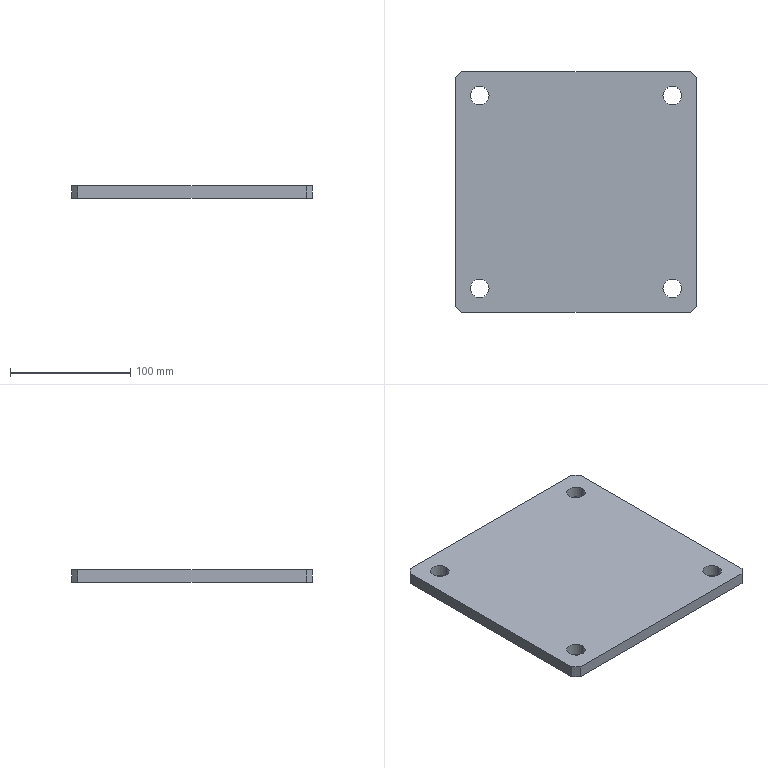Part | NX | features BREP 1 | 1 solid | 18 faces | box 200 x 200 x 10 mm | volume 391952 mm3 | plane 10 | cylinder 8 | commonest cylinder face diameters 15.5 x8
STEP:
#1=CARTESIAN_POINT('',(87.75,80.,0.));
#2=VERTEX_POINT('',#1);
#3=CARTESIAN_POINT('',(72.25,80.,0.));
#4=VERTEX_POINT('',#3);
#5=CARTESIAN_POINT('',(80.,80.,0.));
#6=DIRECTION('',(0.,0.,-1.));
#7=DIRECTION('',(-1.,0.,0.));
#8=AXIS2_PLACEMENT_3D('',#5,#6,#7);
#9=CIRCLE('',#8,7.75);
#10=EDGE_CURVE('',#2,#4,#9,.T.);
#11=ORIENTED_EDGE('',*,*,#10,.T.);
#12=CARTESIAN_POINT('',(72.25,80.,10.));
#13=VERTEX_POINT('',#12);
#14=CARTESIAN_POINT('',(72.25,80.,10.));
#15=DIRECTION('',(0.,0.,1.));
#16=VECTOR('',#15,1000.);
#17=LINE('',#14,#16);
#18=EDGE_CURVE('',#13,#4,#17,.F.);
#19=ORIENTED_EDGE('',*,*,#18,.F.);
#20=CARTESIAN_POINT('',(87.75,80.,10.));
#21=VERTEX_POINT('',#20);
#22=CARTESIAN_POINT('',(80.,80.,10.));
#23=DIRECTION('',(0.,0.,1.));
#24=DIRECTION('',(1.,0.,0.));
#25=AXIS2_PLACEMENT_3D('',#22,#23,#24);
#26=CIRCLE('',#25,7.75);
#27=EDGE_CURVE('',#13,#21,#26,.T.);
#28=ORIENTED_EDGE('',*,*,#27,.T.);
#29=CARTESIAN_POINT('',(87.75,80.,10.));
#30=DIRECTION('',(0.,0.,1.));
#31=VECTOR('',#30,1000.);
#32=LINE('',#29,#31);
#33=EDGE_CURVE('',#21,#2,#32,.F.);
#34=ORIENTED_EDGE('',*,*,#33,.T.);
#35=EDGE_LOOP('',(#11,#19,#28,#34));
#36=FACE_BOUND('',#35,.T.);
#37=CARTESIAN_POINT('',(80.,80.,10.));
#38=DIRECTION('',(0.,0.,1.));
#39=DIRECTION('',(1.,0.,0.));
#40=AXIS2_PLACEMENT_3D('',#37,#38,#39);
#41=CYLINDRICAL_SURFACE('',#40,7.75);
#42=ADVANCED_FACE('',(#36),#41,.F.);
#43=CARTESIAN_POINT('',(-72.25,80.,0.));
#44=VERTEX_POINT('',#43);
#45=CARTESIAN_POINT('',(-87.75,80.,0.));
#46=VERTEX_POINT('',#45);
#47=CARTESIAN_POINT('',(-80.,80.,0.));
#48=DIRECTION('',(0.,0.,-1.));
#49=DIRECTION('',(-1.,0.,0.));
#50=AXIS2_PLACEMENT_3D('',#47,#48,#49);
#51=CIRCLE('',#50,7.75);
#52=EDGE_CURVE('',#44,#46,#51,.T.);
#53=ORIENTED_EDGE('',*,*,#52,.T.);
#54=CARTESIAN_POINT('',(-87.75,80.,10.));
#55=VERTEX_POINT('',#54);
#56=CARTESIAN_POINT('',(-87.75,80.,10.));
#57=DIRECTION('',(0.,0.,1.));
#58=VECTOR('',#57,1000.);
#59=LINE('',#56,#58);
#60=EDGE_CURVE('',#55,#46,#59,.F.);
#61=ORIENTED_EDGE('',*,*,#60,.F.);
#62=CARTESIAN_POINT('',(-72.25,80.,10.));
#63=VERTEX_POINT('',#62);
#64=CARTESIAN_POINT('',(-80.,80.,10.));
#65=DIRECTION('',(0.,0.,1.));
#66=DIRECTION('',(1.,0.,0.));
#67=AXIS2_PLACEMENT_3D('',#64,#65,#66);
#68=CIRCLE('',#67,7.75);
#69=EDGE_CURVE('',#55,#63,#68,.T.);
#70=ORIENTED_EDGE('',*,*,#69,.T.);
#71=CARTESIAN_POINT('',(-72.25,80.,10.));
#72=DIRECTION('',(0.,0.,1.));
#73=VECTOR('',#72,1000.);
#74=LINE('',#71,#73);
#75=EDGE_CURVE('',#63,#44,#74,.F.);
#76=ORIENTED_EDGE('',*,*,#75,.T.);
#77=EDGE_LOOP('',(#53,#61,#70,#76));
#78=FACE_BOUND('',#77,.T.);
#79=CARTESIAN_POINT('',(-80.,80.,10.));
#80=DIRECTION('',(0.,0.,1.));
#81=DIRECTION('',(1.,0.,0.));
#82=AXIS2_PLACEMENT_3D('',#79,#80,#81);
#83=CYLINDRICAL_SURFACE('',#82,7.75);
#84=ADVANCED_FACE('',(#78),#83,.F.);
#85=CARTESIAN_POINT('',(87.75,-80.,0.));
#86=VERTEX_POINT('',#85);
#87=CARTESIAN_POINT('',(72.25,-80.,0.));
#88=VERTEX_POINT('',#87);
#89=CARTESIAN_POINT('',(80.,-80.,0.));
#90=DIRECTION('',(0.,0.,-1.));
#91=DIRECTION('',(-1.,0.,0.));
#92=AXIS2_PLACEMENT_3D('',#89,#90,#91);
#93=CIRCLE('',#92,7.75);
#94=EDGE_CURVE('',#86,#88,#93,.T.);
#95=ORIENTED_EDGE('',*,*,#94,.T.);
#96=CARTESIAN_POINT('',(72.25,-80.,10.));
#97=VERTEX_POINT('',#96);
#98=CARTESIAN_POINT('',(72.25,-80.,10.));
#99=DIRECTION('',(0.,0.,1.));
#100=VECTOR('',#99,1000.);
#101=LINE('',#98,#100);
#102=EDGE_CURVE('',#97,#88,#101,.F.);
#103=ORIENTED_EDGE('',*,*,#102,.F.);
#104=CARTESIAN_POINT('',(87.75,-80.,10.));
#105=VERTEX_POINT('',#104);
#106=CARTESIAN_POINT('',(80.,-80.,10.));
#107=DIRECTION('',(0.,0.,1.));
#108=DIRECTION('',(1.,0.,0.));
#109=AXIS2_PLACEMENT_3D('',#106,#107,#108);
#110=CIRCLE('',#109,7.75);
#111=EDGE_CURVE('',#97,#105,#110,.T.);
#112=ORIENTED_EDGE('',*,*,#111,.T.);
#113=CARTESIAN_POINT('',(87.75,-80.,10.));
#114=DIRECTION('',(0.,0.,1.));
#115=VECTOR('',#114,1000.);
#116=LINE('',#113,#115);
#117=EDGE_CURVE('',#105,#86,#116,.F.);
#118=ORIENTED_EDGE('',*,*,#117,.T.);
#119=EDGE_LOOP('',(#95,#103,#112,#118));
#120=FACE_BOUND('',#119,.T.);
#121=CARTESIAN_POINT('',(80.,-80.,10.));
#122=DIRECTION('',(0.,0.,1.));
#123=DIRECTION('',(1.,0.,0.));
#124=AXIS2_PLACEMENT_3D('',#121,#122,#123);
#125=CYLINDRICAL_SURFACE('',#124,7.75);
#126=ADVANCED_FACE('',(#120),#125,.F.);
#127=CARTESIAN_POINT('',(-72.25,-80.,0.));
#128=VERTEX_POINT('',#127);
#129=CARTESIAN_POINT('',(-87.75,-80.,0.));
#130=VERTEX_POINT('',#129);
#131=CARTESIAN_POINT('',(-80.,-80.,0.));
#132=DIRECTION('',(0.,0.,-1.));
#133=DIRECTION('',(-1.,0.,0.));
#134=AXIS2_PLACEMENT_3D('',#131,#132,#133);
#135=CIRCLE('',#134,7.75);
#136=EDGE_CURVE('',#128,#130,#135,.T.);
#137=ORIENTED_EDGE('',*,*,#136,.T.);
#138=CARTESIAN_POINT('',(-87.75,-80.,10.));
#139=VERTEX_POINT('',#138);
#140=CARTESIAN_POINT('',(-87.75,-80.,10.));
#141=DIRECTION('',(0.,0.,1.));
#142=VECTOR('',#141,1000.);
#143=LINE('',#140,#142);
#144=EDGE_CURVE('',#139,#130,#143,.F.);
#145=ORIENTED_EDGE('',*,*,#144,.F.);
#146=CARTESIAN_POINT('',(-72.25,-80.,10.));
#147=VERTEX_POINT('',#146);
#148=CARTESIAN_POINT('',(-80.,-80.,10.));
#149=DIRECTION('',(0.,0.,1.));
#150=DIRECTION('',(1.,0.,0.));
#151=AXIS2_PLACEMENT_3D('',#148,#149,#150);
#152=CIRCLE('',#151,7.75);
#153=EDGE_CURVE('',#139,#147,#152,.T.);
#154=ORIENTED_EDGE('',*,*,#153,.T.);
#155=CARTESIAN_POINT('',(-72.25,-80.,10.));
#156=DIRECTION('',(0.,0.,1.));
#157=VECTOR('',#156,1000.);
#158=LINE('',#155,#157);
#159=EDGE_CURVE('',#147,#128,#158,.F.);
#160=ORIENTED_EDGE('',*,*,#159,.T.);
#161=EDGE_LOOP('',(#137,#145,#154,#160));
#162=FACE_BOUND('',#161,.T.);
#163=CARTESIAN_POINT('',(-80.,-80.,10.));
#164=DIRECTION('',(0.,0.,1.));
#165=DIRECTION('',(1.,0.,0.));
#166=AXIS2_PLACEMENT_3D('',#163,#164,#165);
#167=CYLINDRICAL_SURFACE('',#166,7.75);
#168=ADVANCED_FACE('',(#162),#167,.F.);
#169=CARTESIAN_POINT('',(100.,-95.,0.));
#170=VERTEX_POINT('',#169);
#171=CARTESIAN_POINT('',(100.,95.,0.));
#172=VERTEX_POINT('',#171);
#173=CARTESIAN_POINT('',(100.,-100.,0.));
#174=DIRECTION('',(0.,1.,0.));
#175=VECTOR('',#174,1000.);
#176=LINE('',#173,#175);
#177=EDGE_CURVE('',#170,#172,#176,.T.);
#178=ORIENTED_EDGE('',*,*,#177,.T.);
#179=CARTESIAN_POINT('',(100.,95.,10.));
#180=VERTEX_POINT('',#179);
#181=CARTESIAN_POINT('',(100.,95.,10.));
#182=DIRECTION('',(0.,0.,1.));
#183=VECTOR('',#182,1000.);
#184=LINE('',#181,#183);
#185=EDGE_CURVE('',#172,#180,#184,.T.);
#186=ORIENTED_EDGE('',*,*,#185,.T.);
#187=CARTESIAN_POINT('',(100.,-95.,10.));
#188=VERTEX_POINT('',#187);
#189=CARTESIAN_POINT('',(100.,-100.,10.));
#190=DIRECTION('',(0.,1.,0.));
#191=VECTOR('',#190,1000.);
#192=LINE('',#189,#191);
#193=EDGE_CURVE('',#188,#180,#192,.T.);
#194=ORIENTED_EDGE('',*,*,#193,.F.);
#195=CARTESIAN_POINT('',(100.,-95.,10.));
#196=DIRECTION('',(0.,0.,-1.));
#197=VECTOR('',#196,1000.);
#198=LINE('',#195,#197);
#199=EDGE_CURVE('',#188,#170,#198,.T.);
#200=ORIENTED_EDGE('',*,*,#199,.T.);
#201=EDGE_LOOP('',(#178,#186,#194,#200));
#202=FACE_BOUND('',#201,.T.);
#203=CARTESIAN_POINT('',(100.,-100.,10.));
#204=DIRECTION('',(-1.,0.,0.));
#205=DIRECTION('',(0.,0.,1.));
#206=AXIS2_PLACEMENT_3D('',#203,#204,#205);
#207=PLANE('',#206);
#208=ADVANCED_FACE('',(#202),#207,.F.);
#209=CARTESIAN_POINT('',(95.,100.,0.));
#210=VERTEX_POINT('',#209);
#211=CARTESIAN_POINT('',(-95.,100.,0.));
#212=VERTEX_POINT('',#211);
#213=CARTESIAN_POINT('',(-100.,100.,0.));
#214=DIRECTION('',(-1.,0.,0.));
#215=VECTOR('',#214,1000.);
#216=LINE('',#213,#215);
#217=EDGE_CURVE('',#210,#212,#216,.T.);
#218=ORIENTED_EDGE('',*,*,#217,.T.);
#219=CARTESIAN_POINT('',(-95.,100.,10.));
#220=VERTEX_POINT('',#219);
#221=CARTESIAN_POINT('',(-95.,100.,10.));
#222=DIRECTION('',(0.,0.,1.));
#223=VECTOR('',#222,1000.);
#224=LINE('',#221,#223);
#225=EDGE_CURVE('',#212,#220,#224,.T.);
#226=ORIENTED_EDGE('',*,*,#225,.T.);
#227=CARTESIAN_POINT('',(95.,100.,10.));
#228=VERTEX_POINT('',#227);
#229=CARTESIAN_POINT('',(-100.,100.,10.));
#230=DIRECTION('',(-1.,0.,0.));
#231=VECTOR('',#230,1000.);
#232=LINE('',#229,#231);
#233=EDGE_CURVE('',#228,#220,#232,.T.);
#234=ORIENTED_EDGE('',*,*,#233,.F.);
#235=CARTESIAN_POINT('',(95.,100.,10.));
#236=DIRECTION('',(0.,0.,-1.));
#237=VECTOR('',#236,1000.);
#238=LINE('',#235,#237);
#239=EDGE_CURVE('',#228,#210,#238,.T.);
#240=ORIENTED_EDGE('',*,*,#239,.T.);
#241=EDGE_LOOP('',(#218,#226,#234,#240));
#242=FACE_BOUND('',#241,.T.);
#243=CARTESIAN_POINT('',(-100.,100.,10.));
#244=DIRECTION('',(0.,-1.,0.));
#245=DIRECTION('',(0.,0.,-1.));
#246=AXIS2_PLACEMENT_3D('',#243,#244,#245);
#247=PLANE('',#246);
#248=ADVANCED_FACE('',(#242),#247,.F.);
#249=CARTESIAN_POINT('',(-100.,95.,10.));
#250=VERTEX_POINT('',#249);
#251=CARTESIAN_POINT('',(-100.,-95.,10.));
#252=VERTEX_POINT('',#251);
#253=CARTESIAN_POINT('',(-100.,-100.,10.));
#254=DIRECTION('',(0.,-1.,0.));
#255=VECTOR('',#254,1000.);
#256=LINE('',#253,#255);
#257=EDGE_CURVE('',#250,#252,#256,.T.);
#258=ORIENTED_EDGE('',*,*,#257,.F.);
#259=CARTESIAN_POINT('',(-100.,95.,0.));
#260=VERTEX_POINT('',#259);
#261=CARTESIAN_POINT('',(-100.,95.,10.));
#262=DIRECTION('',(0.,0.,-1.));
#263=VECTOR('',#262,1000.);
#264=LINE('',#261,#263);
#265=EDGE_CURVE('',#250,#260,#264,.T.);
#266=ORIENTED_EDGE('',*,*,#265,.T.);
#267=CARTESIAN_POINT('',(-100.,-95.,0.));
#268=VERTEX_POINT('',#267);
#269=CARTESIAN_POINT('',(-100.,-100.,0.));
#270=DIRECTION('',(0.,-1.,0.));
#271=VECTOR('',#270,1000.);
#272=LINE('',#269,#271);
#273=EDGE_CURVE('',#260,#268,#272,.T.);
#274=ORIENTED_EDGE('',*,*,#273,.T.);
#275=CARTESIAN_POINT('',(-100.,-95.,10.));
#276=DIRECTION('',(0.,0.,1.));
#277=VECTOR('',#276,1000.);
#278=LINE('',#275,#277);
#279=EDGE_CURVE('',#268,#252,#278,.T.);
#280=ORIENTED_EDGE('',*,*,#279,.T.);
#281=EDGE_LOOP('',(#258,#266,#274,#280));
#282=FACE_BOUND('',#281,.T.);
#283=CARTESIAN_POINT('',(-100.,-100.,10.));
#284=DIRECTION('',(1.,0.,0.));
#285=DIRECTION('',(0.,1.,0.));
#286=AXIS2_PLACEMENT_3D('',#283,#284,#285);
#287=PLANE('',#286);
#288=ADVANCED_FACE('',(#282),#287,.F.);
#289=CARTESIAN_POINT('',(-95.,-100.,0.));
#290=VERTEX_POINT('',#289);
#291=CARTESIAN_POINT('',(95.,-100.,0.));
#292=VERTEX_POINT('',#291);
#293=CARTESIAN_POINT('',(-100.,-100.,0.));
#294=DIRECTION('',(1.,0.,0.));
#295=VECTOR('',#294,1000.);
#296=LINE('',#293,#295);
#297=EDGE_CURVE('',#290,#292,#296,.T.);
#298=ORIENTED_EDGE('',*,*,#297,.T.);
#299=CARTESIAN_POINT('',(95.,-100.,10.));
#300=VERTEX_POINT('',#299);
#301=CARTESIAN_POINT('',(95.,-100.,10.));
#302=DIRECTION('',(0.,0.,1.));
#303=VECTOR('',#302,1000.);
#304=LINE('',#301,#303);
#305=EDGE_CURVE('',#292,#300,#304,.T.);
#306=ORIENTED_EDGE('',*,*,#305,.T.);
#307=CARTESIAN_POINT('',(-95.,-100.,10.));
#308=VERTEX_POINT('',#307);
#309=CARTESIAN_POINT('',(-100.,-100.,10.));
#310=DIRECTION('',(1.,0.,0.));
#311=VECTOR('',#310,1000.);
#312=LINE('',#309,#311);
#313=EDGE_CURVE('',#308,#300,#312,.T.);
#314=ORIENTED_EDGE('',*,*,#313,.F.);
#315=CARTESIAN_POINT('',(-95.,-100.,10.));
#316=DIRECTION('',(0.,0.,-1.));
#317=VECTOR('',#316,1000.);
#318=LINE('',#315,#317);
#319=EDGE_CURVE('',#308,#290,#318,.T.);
#320=ORIENTED_EDGE('',*,*,#319,.T.);
#321=EDGE_LOOP('',(#298,#306,#314,#320));
#322=FACE_BOUND('',#321,.T.);
#323=CARTESIAN_POINT('',(-100.,-100.,10.));
#324=DIRECTION('',(0.,1.,0.));
#325=DIRECTION('',(1.,0.,0.));
#326=AXIS2_PLACEMENT_3D('',#323,#324,#325);
#327=PLANE('',#326);
#328=ADVANCED_FACE('',(#322),#327,.F.);
#329=ORIENTED_EDGE('',*,*,#233,.T.);
#330=CARTESIAN_POINT('',(-100.,95.,10.));
#331=DIRECTION('',(-0.7071,-0.7071,0.));
#332=VECTOR('',#331,1000.);
#333=LINE('',#330,#332);
#334=EDGE_CURVE('',#220,#250,#333,.T.);
#335=ORIENTED_EDGE('',*,*,#334,.T.);
#336=ORIENTED_EDGE('',*,*,#257,.T.);
#337=CARTESIAN_POINT('',(-95.,-100.,10.));
#338=DIRECTION('',(0.7071,-0.7071,0.));
#339=VECTOR('',#338,1000.);
#340=LINE('',#337,#339);
#341=EDGE_CURVE('',#252,#308,#340,.T.);
#342=ORIENTED_EDGE('',*,*,#341,.T.);
#343=ORIENTED_EDGE('',*,*,#313,.T.);
#344=CARTESIAN_POINT('',(100.,-95.,10.));
#345=DIRECTION('',(0.7071,0.7071,0.));
#346=VECTOR('',#345,1000.);
#347=LINE('',#344,#346);
#348=EDGE_CURVE('',#300,#188,#347,.T.);
#349=ORIENTED_EDGE('',*,*,#348,.T.);
#350=ORIENTED_EDGE('',*,*,#193,.T.);
#351=CARTESIAN_POINT('',(95.,100.,10.));
#352=DIRECTION('',(-0.7071,0.7071,0.));
#353=VECTOR('',#352,1000.);
#354=LINE('',#351,#353);
#355=EDGE_CURVE('',#180,#228,#354,.T.);
#356=ORIENTED_EDGE('',*,*,#355,.T.);
#357=EDGE_LOOP('',(#329,#335,#336,#342,#343,#349,#350,#356));
#358=FACE_BOUND('',#357,.T.);
#359=CARTESIAN_POINT('',(80.,80.,10.));
#360=DIRECTION('',(0.,0.,1.));
#361=DIRECTION('',(1.,0.,0.));
#362=AXIS2_PLACEMENT_3D('',#359,#360,#361);
#363=CIRCLE('',#362,7.75);
#364=EDGE_CURVE('',#21,#13,#363,.T.);
#365=ORIENTED_EDGE('',*,*,#364,.F.);
#366=ORIENTED_EDGE('',*,*,#27,.F.);
#367=EDGE_LOOP('',(#365,#366));
#368=FACE_BOUND('',#367,.T.);
#369=CARTESIAN_POINT('',(-80.,80.,10.));
#370=DIRECTION('',(0.,0.,1.));
#371=DIRECTION('',(1.,0.,0.));
#372=AXIS2_PLACEMENT_3D('',#369,#370,#371);
#373=CIRCLE('',#372,7.75);
#374=EDGE_CURVE('',#63,#55,#373,.T.);
#375=ORIENTED_EDGE('',*,*,#374,.F.);
#376=ORIENTED_EDGE('',*,*,#69,.F.);
#377=EDGE_LOOP('',(#375,#376));
#378=FACE_BOUND('',#377,.T.);
#379=CARTESIAN_POINT('',(80.,-80.,10.));
#380=DIRECTION('',(0.,0.,1.));
#381=DIRECTION('',(1.,0.,0.));
#382=AXIS2_PLACEMENT_3D('',#379,#380,#381);
#383=CIRCLE('',#382,7.75);
#384=EDGE_CURVE('',#105,#97,#383,.T.);
#385=ORIENTED_EDGE('',*,*,#384,.F.);
#386=ORIENTED_EDGE('',*,*,#111,.F.);
#387=EDGE_LOOP('',(#385,#386));
#388=FACE_BOUND('',#387,.T.);
#389=CARTESIAN_POINT('',(-80.,-80.,10.));
#390=DIRECTION('',(0.,0.,1.));
#391=DIRECTION('',(1.,0.,0.));
#392=AXIS2_PLACEMENT_3D('',#389,#390,#391);
#393=CIRCLE('',#392,7.75);
#394=EDGE_CURVE('',#147,#139,#393,.T.);
#395=ORIENTED_EDGE('',*,*,#394,.F.);
#396=ORIENTED_EDGE('',*,*,#153,.F.);
#397=EDGE_LOOP('',(#395,#396));
#398=FACE_BOUND('',#397,.T.);
#399=CARTESIAN_POINT('',(0.,0.,10.));
#400=DIRECTION('',(0.,0.,-1.));
#401=DIRECTION('',(0.,-1.,0.));
#402=AXIS2_PLACEMENT_3D('',#399,#400,#401);
#403=PLANE('',#402);
#404=ADVANCED_FACE('',(#358,#368,#378,#388,#398),#403,.F.);
#405=ORIENTED_EDGE('',*,*,#273,.F.);
#406=CARTESIAN_POINT('',(-97.5,97.5,0.));
#407=DIRECTION('',(0.7071,0.7071,0.));
#408=VECTOR('',#407,1000.);
#409=LINE('',#406,#408);
#410=EDGE_CURVE('',#260,#212,#409,.T.);
#411=ORIENTED_EDGE('',*,*,#410,.T.);
#412=ORIENTED_EDGE('',*,*,#217,.F.);
#413=CARTESIAN_POINT('',(97.5,97.5,0.));
#414=DIRECTION('',(0.7071,-0.7071,0.));
#415=VECTOR('',#414,1000.);
#416=LINE('',#413,#415);
#417=EDGE_CURVE('',#210,#172,#416,.T.);
#418=ORIENTED_EDGE('',*,*,#417,.T.);
#419=ORIENTED_EDGE('',*,*,#177,.F.);
#420=CARTESIAN_POINT('',(97.5,-97.5,0.));
#421=DIRECTION('',(-0.7071,-0.7071,0.));
#422=VECTOR('',#421,1000.);
#423=LINE('',#420,#422);
#424=EDGE_CURVE('',#170,#292,#423,.T.);
#425=ORIENTED_EDGE('',*,*,#424,.T.);
#426=ORIENTED_EDGE('',*,*,#297,.F.);
#427=CARTESIAN_POINT('',(-97.5,-97.5,0.));
#428=DIRECTION('',(-0.7071,0.7071,0.));
#429=VECTOR('',#428,1000.);
#430=LINE('',#427,#429);
#431=EDGE_CURVE('',#290,#268,#430,.T.);
#432=ORIENTED_EDGE('',*,*,#431,.T.);
#433=EDGE_LOOP('',(#405,#411,#412,#418,#419,#425,#426,#432));
#434=FACE_BOUND('',#433,.T.);
#435=ORIENTED_EDGE('',*,*,#10,.F.);
#436=CARTESIAN_POINT('',(80.,80.,0.));
#437=DIRECTION('',(0.,0.,-1.));
#438=DIRECTION('',(-1.,0.,0.));
#439=AXIS2_PLACEMENT_3D('',#436,#437,#438);
#440=CIRCLE('',#439,7.75);
#441=EDGE_CURVE('',#4,#2,#440,.T.);
#442=ORIENTED_EDGE('',*,*,#441,.F.);
#443=EDGE_LOOP('',(#435,#442));
#444=FACE_BOUND('',#443,.T.);
#445=ORIENTED_EDGE('',*,*,#52,.F.);
#446=CARTESIAN_POINT('',(-80.,80.,0.));
#447=DIRECTION('',(0.,0.,-1.));
#448=DIRECTION('',(-1.,0.,0.));
#449=AXIS2_PLACEMENT_3D('',#446,#447,#448);
#450=CIRCLE('',#449,7.75);
#451=EDGE_CURVE('',#46,#44,#450,.T.);
#452=ORIENTED_EDGE('',*,*,#451,.F.);
#453=EDGE_LOOP('',(#445,#452));
#454=FACE_BOUND('',#453,.T.);
#455=ORIENTED_EDGE('',*,*,#94,.F.);
#456=CARTESIAN_POINT('',(80.,-80.,0.));
#457=DIRECTION('',(0.,0.,-1.));
#458=DIRECTION('',(-1.,0.,0.));
#459=AXIS2_PLACEMENT_3D('',#456,#457,#458);
#460=CIRCLE('',#459,7.75);
#461=EDGE_CURVE('',#88,#86,#460,.T.);
#462=ORIENTED_EDGE('',*,*,#461,.F.);
#463=EDGE_LOOP('',(#455,#462));
#464=FACE_BOUND('',#463,.T.);
#465=ORIENTED_EDGE('',*,*,#136,.F.);
#466=CARTESIAN_POINT('',(-80.,-80.,0.));
#467=DIRECTION('',(0.,0.,-1.));
#468=DIRECTION('',(-1.,0.,0.));
#469=AXIS2_PLACEMENT_3D('',#466,#467,#468);
#470=CIRCLE('',#469,7.75);
#471=EDGE_CURVE('',#130,#128,#470,.T.);
#472=ORIENTED_EDGE('',*,*,#471,.F.);
#473=EDGE_LOOP('',(#465,#472));
#474=FACE_BOUND('',#473,.T.);
#475=CARTESIAN_POINT('',(0.,0.,0.));
#476=DIRECTION('',(0.,0.,-1.));
#477=DIRECTION('',(0.,-1.,0.));
#478=AXIS2_PLACEMENT_3D('',#475,#476,#477);
#479=PLANE('',#478);
#480=ADVANCED_FACE('',(#434,#444,#454,#464,#474),#479,.T.);
#481=ORIENTED_EDGE('',*,*,#144,.T.);
#482=ORIENTED_EDGE('',*,*,#471,.T.);
#483=ORIENTED_EDGE('',*,*,#159,.F.);
#484=ORIENTED_EDGE('',*,*,#394,.T.);
#485=EDGE_LOOP('',(#481,#482,#483,#484));
#486=FACE_BOUND('',#485,.T.);
#487=CARTESIAN_POINT('',(-80.,-80.,10.));
#488=DIRECTION('',(0.,0.,1.));
#489=DIRECTION('',(1.,0.,0.));
#490=AXIS2_PLACEMENT_3D('',#487,#488,#489);
#491=CYLINDRICAL_SURFACE('',#490,7.75);
#492=ADVANCED_FACE('',(#486),#491,.F.);
#493=ORIENTED_EDGE('',*,*,#102,.T.);
#494=ORIENTED_EDGE('',*,*,#461,.T.);
#495=ORIENTED_EDGE('',*,*,#117,.F.);
#496=ORIENTED_EDGE('',*,*,#384,.T.);
#497=EDGE_LOOP('',(#493,#494,#495,#496));
#498=FACE_BOUND('',#497,.T.);
#499=CARTESIAN_POINT('',(80.,-80.,10.));
#500=DIRECTION('',(0.,0.,1.));
#501=DIRECTION('',(1.,0.,0.));
#502=AXIS2_PLACEMENT_3D('',#499,#500,#501);
#503=CYLINDRICAL_SURFACE('',#502,7.75);
#504=ADVANCED_FACE('',(#498),#503,.F.);
#505=ORIENTED_EDGE('',*,*,#60,.T.);
#506=ORIENTED_EDGE('',*,*,#451,.T.);
#507=ORIENTED_EDGE('',*,*,#75,.F.);
#508=ORIENTED_EDGE('',*,*,#374,.T.);
#509=EDGE_LOOP('',(#505,#506,#507,#508));
#510=FACE_BOUND('',#509,.T.);
#511=CARTESIAN_POINT('',(-80.,80.,10.));
#512=DIRECTION('',(0.,0.,1.));
#513=DIRECTION('',(1.,0.,0.));
#514=AXIS2_PLACEMENT_3D('',#511,#512,#513);
#515=CYLINDRICAL_SURFACE('',#514,7.75);
#516=ADVANCED_FACE('',(#510),#515,.F.);
#517=ORIENTED_EDGE('',*,*,#18,.T.);
#518=ORIENTED_EDGE('',*,*,#441,.T.);
#519=ORIENTED_EDGE('',*,*,#33,.F.);
#520=ORIENTED_EDGE('',*,*,#364,.T.);
#521=EDGE_LOOP('',(#517,#518,#519,#520));
#522=FACE_BOUND('',#521,.T.);
#523=CARTESIAN_POINT('',(80.,80.,10.));
#524=DIRECTION('',(0.,0.,1.));
#525=DIRECTION('',(1.,0.,0.));
#526=AXIS2_PLACEMENT_3D('',#523,#524,#525);
#527=CYLINDRICAL_SURFACE('',#526,7.75);
#528=ADVANCED_FACE('',(#522),#527,.F.);
#529=ORIENTED_EDGE('',*,*,#334,.F.);
#530=ORIENTED_EDGE('',*,*,#225,.F.);
#531=ORIENTED_EDGE('',*,*,#410,.F.);
#532=ORIENTED_EDGE('',*,*,#265,.F.);
#533=EDGE_LOOP('',(#529,#530,#531,#532));
#534=FACE_BOUND('',#533,.T.);
#535=CARTESIAN_POINT('',(-100.,95.,10.));
#536=DIRECTION('',(0.7071,-0.7071,0.));
#537=DIRECTION('',(0.,0.,-1.));
#538=AXIS2_PLACEMENT_3D('',#535,#536,#537);
#539=PLANE('',#538);
#540=ADVANCED_FACE('',(#534),#539,.F.);
#541=ORIENTED_EDGE('',*,*,#355,.F.);
#542=ORIENTED_EDGE('',*,*,#185,.F.);
#543=ORIENTED_EDGE('',*,*,#417,.F.);
#544=ORIENTED_EDGE('',*,*,#239,.F.);
#545=EDGE_LOOP('',(#541,#542,#543,#544));
#546=FACE_BOUND('',#545,.T.);
#547=CARTESIAN_POINT('',(95.,100.,10.));
#548=DIRECTION('',(-0.7071,-0.7071,0.));
#549=DIRECTION('',(-0.7071,0.7071,0.));
#550=AXIS2_PLACEMENT_3D('',#547,#548,#549);
#551=PLANE('',#550);
#552=ADVANCED_FACE('',(#546),#551,.F.);
#553=ORIENTED_EDGE('',*,*,#348,.F.);
#554=ORIENTED_EDGE('',*,*,#305,.F.);
#555=ORIENTED_EDGE('',*,*,#424,.F.);
#556=ORIENTED_EDGE('',*,*,#199,.F.);
#557=EDGE_LOOP('',(#553,#554,#555,#556));
#558=FACE_BOUND('',#557,.T.);
#559=CARTESIAN_POINT('',(100.,-95.,10.));
#560=DIRECTION('',(-0.7071,0.7071,0.));
#561=DIRECTION('',(0.,0.,1.));
#562=AXIS2_PLACEMENT_3D('',#559,#560,#561);
#563=PLANE('',#562);
#564=ADVANCED_FACE('',(#558),#563,.F.);
#565=ORIENTED_EDGE('',*,*,#341,.F.);
#566=ORIENTED_EDGE('',*,*,#279,.F.);
#567=ORIENTED_EDGE('',*,*,#431,.F.);
#568=ORIENTED_EDGE('',*,*,#319,.F.);
#569=EDGE_LOOP('',(#565,#566,#567,#568));
#570=FACE_BOUND('',#569,.T.);
#571=CARTESIAN_POINT('',(-95.,-100.,10.));
#572=DIRECTION('',(0.7071,0.7071,0.));
#573=DIRECTION('',(0.,0.,-1.));
#574=AXIS2_PLACEMENT_3D('',#571,#572,#573);
#575=PLANE('',#574);
#576=ADVANCED_FACE('',(#570),#575,.F.);
#577=CLOSED_SHELL('',(#42,#84,#126,#168,#208,#248,#288,#328,#404,#480,#492,#504,#516,#528,#540,#552,#564,#576));
#578=MANIFOLD_SOLID_BREP('',#577);
#579=(LENGTH_UNIT()NAMED_UNIT(*)SI_UNIT(.MILLI.,.METRE.));
#580=UNCERTAINTY_MEASURE_WITH_UNIT(LENGTH_MEASURE(0.00001),#579,'','');
#581=(NAMED_UNIT(*)PLANE_ANGLE_UNIT()SI_UNIT($,.RADIAN.));
#582=(NAMED_UNIT(*)SI_UNIT($,.STERADIAN.)SOLID_ANGLE_UNIT());
#583=(GEOMETRIC_REPRESENTATION_CONTEXT(3)GLOBAL_UNCERTAINTY_ASSIGNED_CONTEXT((#580))GLOBAL_UNIT_ASSIGNED_CONTEXT((#579,#581,#582))REPRESENTATION_CONTEXT('',''));
#584=ADVANCED_BREP_SHAPE_REPRESENTATION('',(#578),#583);